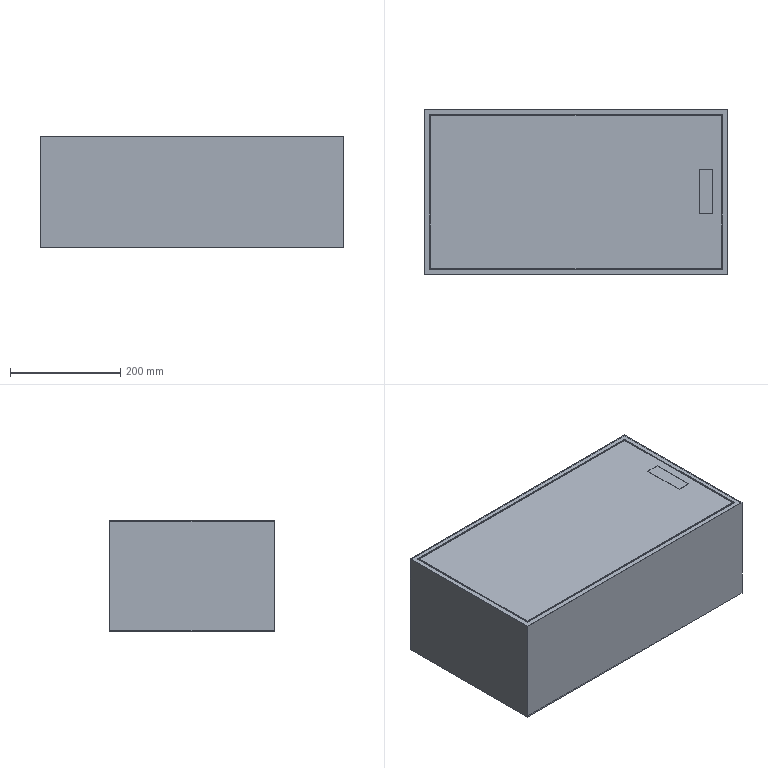Part | SolidWorks | features ICE 3, Extrusion 1, Shell 1 | 1 solid | 38 faces | box 550 x 300 x 201 mm | volume 911866 mm3 | plane 34 | cylinder 4 | commonest cylinder face diameters 22 x4
STEP:
#1=CARTESIAN_POINT('',(549.5,110.,154.));
#2=VERTEX_POINT('',#1);
#3=CARTESIAN_POINT('',(549.5,110.,132.));
#4=VERTEX_POINT('',#3);
#5=CARTESIAN_POINT('',(549.5,110.,143.));
#6=DIRECTION('',(1.,0.,0.));
#7=DIRECTION('',(0.,0.,-1.));
#8=AXIS2_PLACEMENT_3D('',#5,#6,#7);
#9=CIRCLE('',#8,11.);
#10=EDGE_CURVE('',#2,#4,#9,.T.);
#11=ORIENTED_EDGE('',*,*,#10,.F.);
#12=CARTESIAN_POINT('',(550.,110.,154.));
#13=VERTEX_POINT('',#12);
#14=CARTESIAN_POINT('',(549.5,110.,154.));
#15=DIRECTION('',(1.,0.,0.));
#16=VECTOR('',#15,1000.);
#17=LINE('',#14,#16);
#18=EDGE_CURVE('',#2,#13,#17,.T.);
#19=ORIENTED_EDGE('',*,*,#18,.T.);
#20=CARTESIAN_POINT('',(550.,110.,132.));
#21=VERTEX_POINT('',#20);
#22=CARTESIAN_POINT('',(550.,110.,143.));
#23=DIRECTION('',(1.,0.,0.));
#24=DIRECTION('',(0.,0.,-1.));
#25=AXIS2_PLACEMENT_3D('',#22,#23,#24);
#26=CIRCLE('',#25,11.);
#27=EDGE_CURVE('',#13,#21,#26,.T.);
#28=ORIENTED_EDGE('',*,*,#27,.T.);
#29=CARTESIAN_POINT('',(549.5,110.,132.));
#30=DIRECTION('',(1.,0.,0.));
#31=VECTOR('',#30,1000.);
#32=LINE('',#29,#31);
#33=EDGE_CURVE('',#4,#21,#32,.T.);
#34=ORIENTED_EDGE('',*,*,#33,.F.);
#35=EDGE_LOOP('',(#11,#19,#28,#34));
#36=FACE_OUTER_BOUND('',#35,.T.);
#37=CARTESIAN_POINT('',(549.5,110.,143.));
#38=DIRECTION('',(1.,0.,0.));
#39=DIRECTION('',(0.,0.,-1.));
#40=AXIS2_PLACEMENT_3D('',#37,#38,#39);
#41=CYLINDRICAL_SURFACE('',#40,11.);
#42=ADVANCED_FACE('',(#36),#41,.F.);
#43=CARTESIAN_POINT('',(549.5,110.,69.));
#44=VERTEX_POINT('',#43);
#45=CARTESIAN_POINT('',(549.5,110.,47.));
#46=VERTEX_POINT('',#45);
#47=CARTESIAN_POINT('',(549.5,110.,58.));
#48=DIRECTION('',(1.,0.,0.));
#49=DIRECTION('',(0.,0.,-1.));
#50=AXIS2_PLACEMENT_3D('',#47,#48,#49);
#51=CIRCLE('',#50,11.);
#52=EDGE_CURVE('',#44,#46,#51,.T.);
#53=ORIENTED_EDGE('',*,*,#52,.F.);
#54=CARTESIAN_POINT('',(550.,110.,69.));
#55=VERTEX_POINT('',#54);
#56=CARTESIAN_POINT('',(549.5,110.,69.));
#57=DIRECTION('',(1.,0.,0.));
#58=VECTOR('',#57,1000.);
#59=LINE('',#56,#58);
#60=EDGE_CURVE('',#44,#55,#59,.T.);
#61=ORIENTED_EDGE('',*,*,#60,.T.);
#62=CARTESIAN_POINT('',(550.,110.,47.));
#63=VERTEX_POINT('',#62);
#64=CARTESIAN_POINT('',(550.,110.,58.));
#65=DIRECTION('',(1.,0.,0.));
#66=DIRECTION('',(0.,0.,-1.));
#67=AXIS2_PLACEMENT_3D('',#64,#65,#66);
#68=CIRCLE('',#67,11.);
#69=EDGE_CURVE('',#55,#63,#68,.T.);
#70=ORIENTED_EDGE('',*,*,#69,.T.);
#71=CARTESIAN_POINT('',(549.5,110.,47.));
#72=DIRECTION('',(1.,0.,0.));
#73=VECTOR('',#72,1000.);
#74=LINE('',#71,#73);
#75=EDGE_CURVE('',#46,#63,#74,.T.);
#76=ORIENTED_EDGE('',*,*,#75,.F.);
#77=EDGE_LOOP('',(#53,#61,#70,#76));
#78=FACE_OUTER_BOUND('',#77,.T.);
#79=CARTESIAN_POINT('',(549.5,110.,58.));
#80=DIRECTION('',(1.,0.,0.));
#81=DIRECTION('',(0.,0.,-1.));
#82=AXIS2_PLACEMENT_3D('',#79,#80,#81);
#83=CYLINDRICAL_SURFACE('',#82,11.);
#84=ADVANCED_FACE('',(#78),#83,.F.);
#85=CARTESIAN_POINT('',(0.,300.,0.));
#86=VERTEX_POINT('',#85);
#87=CARTESIAN_POINT('',(0.,0.,0.));
#88=VERTEX_POINT('',#87);
#89=CARTESIAN_POINT('',(0.,0.,0.));
#90=DIRECTION('',(0.,-1.,0.));
#91=VECTOR('',#90,1000.);
#92=LINE('',#89,#91);
#93=EDGE_CURVE('',#86,#88,#92,.T.);
#94=ORIENTED_EDGE('',*,*,#93,.T.);
#95=CARTESIAN_POINT('',(0.,0.,201.));
#96=VERTEX_POINT('',#95);
#97=CARTESIAN_POINT('',(0.,0.,200.));
#98=DIRECTION('',(0.,0.,-1.));
#99=VECTOR('',#98,1000.);
#100=LINE('',#97,#99);
#101=EDGE_CURVE('',#96,#88,#100,.T.);
#102=ORIENTED_EDGE('',*,*,#101,.F.);
#103=CARTESIAN_POINT('',(0.,300.,201.));
#104=VERTEX_POINT('',#103);
#105=CARTESIAN_POINT('',(0.,300.,201.));
#106=DIRECTION('',(0.,-1.,0.));
#107=VECTOR('',#106,1000.);
#108=LINE('',#105,#107);
#109=EDGE_CURVE('',#104,#96,#108,.T.);
#110=ORIENTED_EDGE('',*,*,#109,.F.);
#111=CARTESIAN_POINT('',(0.,300.,200.));
#112=DIRECTION('',(0.,0.,-1.));
#113=VECTOR('',#112,1000.);
#114=LINE('',#111,#113);
#115=EDGE_CURVE('',#104,#86,#114,.T.);
#116=ORIENTED_EDGE('',*,*,#115,.T.);
#117=EDGE_LOOP('',(#94,#102,#110,#116));
#118=FACE_OUTER_BOUND('',#117,.T.);
#119=CARTESIAN_POINT('',(0.,0.,200.));
#120=DIRECTION('',(1.,0.,0.));
#121=DIRECTION('',(0.,0.,-1.));
#122=AXIS2_PLACEMENT_3D('',#119,#120,#121);
#123=PLANE('',#122);
#124=ADVANCED_FACE('',(#118),#123,.F.);
#125=CARTESIAN_POINT('',(550.,0.,0.));
#126=VERTEX_POINT('',#125);
#127=CARTESIAN_POINT('',(0.,0.,0.));
#128=DIRECTION('',(1.,0.,0.));
#129=VECTOR('',#128,1000.);
#130=LINE('',#127,#129);
#131=EDGE_CURVE('',#88,#126,#130,.T.);
#132=ORIENTED_EDGE('',*,*,#131,.T.);
#133=CARTESIAN_POINT('',(550.,0.,201.));
#134=VERTEX_POINT('',#133);
#135=CARTESIAN_POINT('',(550.,0.,200.));
#136=DIRECTION('',(0.,0.,-1.));
#137=VECTOR('',#136,1000.);
#138=LINE('',#135,#137);
#139=EDGE_CURVE('',#134,#126,#138,.T.);
#140=ORIENTED_EDGE('',*,*,#139,.F.);
#141=CARTESIAN_POINT('',(0.,0.,201.));
#142=DIRECTION('',(1.,0.,0.));
#143=VECTOR('',#142,1000.);
#144=LINE('',#141,#143);
#145=EDGE_CURVE('',#96,#134,#144,.T.);
#146=ORIENTED_EDGE('',*,*,#145,.F.);
#147=ORIENTED_EDGE('',*,*,#101,.T.);
#148=EDGE_LOOP('',(#132,#140,#146,#147));
#149=FACE_OUTER_BOUND('',#148,.T.);
#150=CARTESIAN_POINT('',(0.,0.,200.));
#151=DIRECTION('',(0.,1.,0.));
#152=DIRECTION('',(0.,0.,1.));
#153=AXIS2_PLACEMENT_3D('',#150,#151,#152);
#154=PLANE('',#153);
#155=ADVANCED_FACE('',(#149),#154,.F.);
#156=CARTESIAN_POINT('',(550.,240.,54.5));
#157=VERTEX_POINT('',#156);
#158=CARTESIAN_POINT('',(550.,240.,146.5));
#159=VERTEX_POINT('',#158);
#160=CARTESIAN_POINT('',(550.,240.,146.5));
#161=DIRECTION('',(0.,0.,1.));
#162=VECTOR('',#161,1000.);
#163=LINE('',#160,#162);
#164=EDGE_CURVE('',#157,#159,#163,.T.);
#165=ORIENTED_EDGE('',*,*,#164,.F.);
#166=CARTESIAN_POINT('',(550.,195.,54.5));
#167=VERTEX_POINT('',#166);
#168=CARTESIAN_POINT('',(550.,240.,54.5));
#169=DIRECTION('',(0.,1.,0.));
#170=VECTOR('',#169,1000.);
#171=LINE('',#168,#170);
#172=EDGE_CURVE('',#167,#157,#171,.T.);
#173=ORIENTED_EDGE('',*,*,#172,.F.);
#174=CARTESIAN_POINT('',(550.,195.,146.5));
#175=VERTEX_POINT('',#174);
#176=CARTESIAN_POINT('',(550.,195.,146.5));
#177=DIRECTION('',(0.,0.,-1.));
#178=VECTOR('',#177,1000.);
#179=LINE('',#176,#178);
#180=EDGE_CURVE('',#175,#167,#179,.T.);
#181=ORIENTED_EDGE('',*,*,#180,.F.);
#182=CARTESIAN_POINT('',(550.,240.,146.5));
#183=DIRECTION('',(0.,-1.,0.));
#184=VECTOR('',#183,1000.);
#185=LINE('',#182,#184);
#186=EDGE_CURVE('',#159,#175,#185,.T.);
#187=ORIENTED_EDGE('',*,*,#186,.F.);
#188=EDGE_LOOP('',(#165,#173,#181,#187));
#189=FACE_BOUND('',#188,.T.);
#190=CARTESIAN_POINT('',(550.,110.,143.));
#191=DIRECTION('',(1.,0.,0.));
#192=DIRECTION('',(0.,0.,-1.));
#193=AXIS2_PLACEMENT_3D('',#190,#191,#192);
#194=CIRCLE('',#193,11.);
#195=EDGE_CURVE('',#21,#13,#194,.T.);
#196=ORIENTED_EDGE('',*,*,#195,.F.);
#197=ORIENTED_EDGE('',*,*,#27,.F.);
#198=EDGE_LOOP('',(#196,#197));
#199=FACE_BOUND('',#198,.T.);
#200=CARTESIAN_POINT('',(550.,110.,58.));
#201=DIRECTION('',(1.,0.,0.));
#202=DIRECTION('',(0.,0.,-1.));
#203=AXIS2_PLACEMENT_3D('',#200,#201,#202);
#204=CIRCLE('',#203,11.);
#205=EDGE_CURVE('',#63,#55,#204,.T.);
#206=ORIENTED_EDGE('',*,*,#205,.F.);
#207=ORIENTED_EDGE('',*,*,#69,.F.);
#208=EDGE_LOOP('',(#206,#207));
#209=FACE_BOUND('',#208,.T.);
#210=CARTESIAN_POINT('',(550.,300.,0.));
#211=VERTEX_POINT('',#210);
#212=CARTESIAN_POINT('',(550.,0.,0.));
#213=DIRECTION('',(0.,1.,0.));
#214=VECTOR('',#213,1000.);
#215=LINE('',#212,#214);
#216=EDGE_CURVE('',#126,#211,#215,.T.);
#217=ORIENTED_EDGE('',*,*,#216,.T.);
#218=CARTESIAN_POINT('',(550.,300.,201.));
#219=VERTEX_POINT('',#218);
#220=CARTESIAN_POINT('',(550.,300.,200.));
#221=DIRECTION('',(0.,0.,-1.));
#222=VECTOR('',#221,1000.);
#223=LINE('',#220,#222);
#224=EDGE_CURVE('',#219,#211,#223,.T.);
#225=ORIENTED_EDGE('',*,*,#224,.F.);
#226=CARTESIAN_POINT('',(550.,0.,201.));
#227=DIRECTION('',(0.,1.,0.));
#228=VECTOR('',#227,1000.);
#229=LINE('',#226,#228);
#230=EDGE_CURVE('',#134,#219,#229,.T.);
#231=ORIENTED_EDGE('',*,*,#230,.F.);
#232=ORIENTED_EDGE('',*,*,#139,.T.);
#233=EDGE_LOOP('',(#217,#225,#231,#232));
#234=FACE_OUTER_BOUND('',#233,.T.);
#235=CARTESIAN_POINT('',(550.,0.,200.));
#236=DIRECTION('',(-1.,0.,0.));
#237=DIRECTION('',(0.,0.,1.));
#238=AXIS2_PLACEMENT_3D('',#235,#236,#237);
#239=PLANE('',#238);
#240=ADVANCED_FACE('',(#189,#199,#209,#234),#239,.F.);
#241=CARTESIAN_POINT('',(0.,300.,0.));
#242=DIRECTION('',(-1.,0.,0.));
#243=VECTOR('',#242,1000.);
#244=LINE('',#241,#243);
#245=EDGE_CURVE('',#211,#86,#244,.T.);
#246=ORIENTED_EDGE('',*,*,#245,.T.);
#247=ORIENTED_EDGE('',*,*,#115,.F.);
#248=CARTESIAN_POINT('',(550.,300.,201.));
#249=DIRECTION('',(-1.,0.,0.));
#250=VECTOR('',#249,1000.);
#251=LINE('',#248,#250);
#252=EDGE_CURVE('',#219,#104,#251,.T.);
#253=ORIENTED_EDGE('',*,*,#252,.F.);
#254=ORIENTED_EDGE('',*,*,#224,.T.);
#255=EDGE_LOOP('',(#246,#247,#253,#254));
#256=FACE_OUTER_BOUND('',#255,.T.);
#257=CARTESIAN_POINT('',(0.,300.,200.));
#258=DIRECTION('',(0.,-1.,0.));
#259=DIRECTION('',(0.,0.,-1.));
#260=AXIS2_PLACEMENT_3D('',#257,#258,#259);
#261=PLANE('',#260);
#262=ADVANCED_FACE('',(#256),#261,.F.);
#263=ORIENTED_EDGE('',*,*,#93,.F.);
#264=ORIENTED_EDGE('',*,*,#245,.F.);
#265=ORIENTED_EDGE('',*,*,#216,.F.);
#266=ORIENTED_EDGE('',*,*,#131,.F.);
#267=EDGE_LOOP('',(#263,#264,#265,#266));
#268=FACE_OUTER_BOUND('',#267,.T.);
#269=CARTESIAN_POINT('',(0.,0.,0.));
#270=DIRECTION('',(0.,0.,-1.));
#271=DIRECTION('',(-1.,0.,0.));
#272=AXIS2_PLACEMENT_3D('',#269,#270,#271);
#273=PLANE('',#272);
#274=ADVANCED_FACE('',(#268),#273,.T.);
#275=CARTESIAN_POINT('',(540.,290.,201.));
#276=VERTEX_POINT('',#275);
#277=CARTESIAN_POINT('',(10.,290.,201.));
#278=VERTEX_POINT('',#277);
#279=CARTESIAN_POINT('',(0.,290.,201.));
#280=DIRECTION('',(-1.,0.,0.));
#281=VECTOR('',#280,1000.);
#282=LINE('',#279,#281);
#283=EDGE_CURVE('',#276,#278,#282,.T.);
#284=ORIENTED_EDGE('',*,*,#283,.F.);
#285=CARTESIAN_POINT('',(540.,10.,201.));
#286=VERTEX_POINT('',#285);
#287=CARTESIAN_POINT('',(540.,0.,201.));
#288=DIRECTION('',(0.,1.,0.));
#289=VECTOR('',#288,1000.);
#290=LINE('',#287,#289);
#291=EDGE_CURVE('',#286,#276,#290,.T.);
#292=ORIENTED_EDGE('',*,*,#291,.F.);
#293=CARTESIAN_POINT('',(10.,10.,201.));
#294=VERTEX_POINT('',#293);
#295=CARTESIAN_POINT('',(0.,10.,201.));
#296=DIRECTION('',(1.,0.,0.));
#297=VECTOR('',#296,1000.);
#298=LINE('',#295,#297);
#299=EDGE_CURVE('',#294,#286,#298,.T.);
#300=ORIENTED_EDGE('',*,*,#299,.F.);
#301=CARTESIAN_POINT('',(10.,0.,201.));
#302=DIRECTION('',(0.,-1.,0.));
#303=VECTOR('',#302,1000.);
#304=LINE('',#301,#303);
#305=EDGE_CURVE('',#278,#294,#304,.T.);
#306=ORIENTED_EDGE('',*,*,#305,.F.);
#307=EDGE_LOOP('',(#284,#292,#300,#306));
#308=FACE_BOUND('',#307,.T.);
#309=ORIENTED_EDGE('',*,*,#252,.T.);
#310=ORIENTED_EDGE('',*,*,#109,.T.);
#311=ORIENTED_EDGE('',*,*,#145,.T.);
#312=ORIENTED_EDGE('',*,*,#230,.T.);
#313=EDGE_LOOP('',(#309,#310,#311,#312));
#314=FACE_OUTER_BOUND('',#313,.T.);
#315=CARTESIAN_POINT('',(0.,0.,201.));
#316=DIRECTION('',(0.,0.,1.));
#317=DIRECTION('',(1.,0.,0.));
#318=AXIS2_PLACEMENT_3D('',#315,#316,#317);
#319=PLANE('',#318);
#320=ADVANCED_FACE('',(#308,#314),#319,.T.);
#321=ORIENTED_EDGE('',*,*,#283,.T.);
#322=CARTESIAN_POINT('',(10.,290.,200.5));
#323=VERTEX_POINT('',#322);
#324=CARTESIAN_POINT('',(10.,290.,200.5));
#325=DIRECTION('',(0.,0.,1.));
#326=VECTOR('',#325,1000.);
#327=LINE('',#324,#326);
#328=EDGE_CURVE('',#323,#278,#327,.T.);
#329=ORIENTED_EDGE('',*,*,#328,.F.);
#330=CARTESIAN_POINT('',(540.,290.,200.5));
#331=VERTEX_POINT('',#330);
#332=CARTESIAN_POINT('',(0.,290.,200.5));
#333=DIRECTION('',(-1.,0.,0.));
#334=VECTOR('',#333,1000.);
#335=LINE('',#332,#334);
#336=EDGE_CURVE('',#331,#323,#335,.T.);
#337=ORIENTED_EDGE('',*,*,#336,.F.);
#338=CARTESIAN_POINT('',(540.,290.,200.5));
#339=DIRECTION('',(0.,0.,1.));
#340=VECTOR('',#339,1000.);
#341=LINE('',#338,#340);
#342=EDGE_CURVE('',#331,#276,#341,.T.);
#343=ORIENTED_EDGE('',*,*,#342,.T.);
#344=EDGE_LOOP('',(#321,#329,#337,#343));
#345=FACE_OUTER_BOUND('',#344,.T.);
#346=CARTESIAN_POINT('',(0.,290.,200.5));
#347=DIRECTION('',(0.,1.,0.));
#348=DIRECTION('',(0.,0.,1.));
#349=AXIS2_PLACEMENT_3D('',#346,#347,#348);
#350=PLANE('',#349);
#351=ADVANCED_FACE('',(#345),#350,.F.);
#352=ORIENTED_EDGE('',*,*,#291,.T.);
#353=ORIENTED_EDGE('',*,*,#342,.F.);
#354=CARTESIAN_POINT('',(540.,10.,200.5));
#355=VERTEX_POINT('',#354);
#356=CARTESIAN_POINT('',(540.,0.,200.5));
#357=DIRECTION('',(0.,1.,0.));
#358=VECTOR('',#357,1000.);
#359=LINE('',#356,#358);
#360=EDGE_CURVE('',#355,#331,#359,.T.);
#361=ORIENTED_EDGE('',*,*,#360,.F.);
#362=CARTESIAN_POINT('',(540.,10.,200.5));
#363=DIRECTION('',(0.,0.,1.));
#364=VECTOR('',#363,1000.);
#365=LINE('',#362,#364);
#366=EDGE_CURVE('',#355,#286,#365,.T.);
#367=ORIENTED_EDGE('',*,*,#366,.T.);
#368=EDGE_LOOP('',(#352,#353,#361,#367));
#369=FACE_OUTER_BOUND('',#368,.T.);
#370=CARTESIAN_POINT('',(540.,0.,200.5));
#371=DIRECTION('',(1.,0.,0.));
#372=DIRECTION('',(0.,0.,-1.));
#373=AXIS2_PLACEMENT_3D('',#370,#371,#372);
#374=PLANE('',#373);
#375=ADVANCED_FACE('',(#369),#374,.F.);
#376=ORIENTED_EDGE('',*,*,#299,.T.);
#377=ORIENTED_EDGE('',*,*,#366,.F.);
#378=CARTESIAN_POINT('',(10.,10.,200.5));
#379=VERTEX_POINT('',#378);
#380=CARTESIAN_POINT('',(0.,10.,200.5));
#381=DIRECTION('',(1.,0.,0.));
#382=VECTOR('',#381,1000.);
#383=LINE('',#380,#382);
#384=EDGE_CURVE('',#379,#355,#383,.T.);
#385=ORIENTED_EDGE('',*,*,#384,.F.);
#386=CARTESIAN_POINT('',(10.,10.,200.5));
#387=DIRECTION('',(0.,0.,1.));
#388=VECTOR('',#387,1000.);
#389=LINE('',#386,#388);
#390=EDGE_CURVE('',#379,#294,#389,.T.);
#391=ORIENTED_EDGE('',*,*,#390,.T.);
#392=EDGE_LOOP('',(#376,#377,#385,#391));
#393=FACE_OUTER_BOUND('',#392,.T.);
#394=CARTESIAN_POINT('',(0.,10.,200.5));
#395=DIRECTION('',(0.,-1.,0.));
#396=DIRECTION('',(0.,0.,-1.));
#397=AXIS2_PLACEMENT_3D('',#394,#395,#396);
#398=PLANE('',#397);
#399=ADVANCED_FACE('',(#393),#398,.F.);
#400=CARTESIAN_POINT('',(538.,12.,201.));
#401=VERTEX_POINT('',#400);
#402=CARTESIAN_POINT('',(538.,288.,201.));
#403=VERTEX_POINT('',#402);
#404=CARTESIAN_POINT('',(538.,0.,201.));
#405=DIRECTION('',(0.,1.,0.));
#406=VECTOR('',#405,1000.);
#407=LINE('',#404,#406);
#408=EDGE_CURVE('',#401,#403,#407,.T.);
#409=ORIENTED_EDGE('',*,*,#408,.F.);
#410=CARTESIAN_POINT('',(538.,12.,200.5));
#411=VERTEX_POINT('',#410);
#412=CARTESIAN_POINT('',(538.,12.,200.5));
#413=DIRECTION('',(0.,0.,1.));
#414=VECTOR('',#413,1000.);
#415=LINE('',#412,#414);
#416=EDGE_CURVE('',#411,#401,#415,.T.);
#417=ORIENTED_EDGE('',*,*,#416,.F.);
#418=CARTESIAN_POINT('',(538.,288.,200.5));
#419=VERTEX_POINT('',#418);
#420=CARTESIAN_POINT('',(538.,0.,200.5));
#421=DIRECTION('',(0.,1.,0.));
#422=VECTOR('',#421,1000.);
#423=LINE('',#420,#422);
#424=EDGE_CURVE('',#411,#419,#423,.T.);
#425=ORIENTED_EDGE('',*,*,#424,.T.);
#426=CARTESIAN_POINT('',(538.,288.,200.5));
#427=DIRECTION('',(0.,0.,1.));
#428=VECTOR('',#427,1000.);
#429=LINE('',#426,#428);
#430=EDGE_CURVE('',#419,#403,#429,.T.);
#431=ORIENTED_EDGE('',*,*,#430,.T.);
#432=EDGE_LOOP('',(#409,#417,#425,#431));
#433=FACE_OUTER_BOUND('',#432,.T.);
#434=CARTESIAN_POINT('',(538.,0.,200.5));
#435=DIRECTION('',(1.,0.,0.));
#436=DIRECTION('',(0.,0.,-1.));
#437=AXIS2_PLACEMENT_3D('',#434,#435,#436);
#438=PLANE('',#437);
#439=ADVANCED_FACE('',(#433),#438,.T.);
#440=CARTESIAN_POINT('',(12.,288.,201.));
#441=VERTEX_POINT('',#440);
#442=CARTESIAN_POINT('',(0.,288.,201.));
#443=DIRECTION('',(-1.,0.,0.));
#444=VECTOR('',#443,1000.);
#445=LINE('',#442,#444);
#446=EDGE_CURVE('',#403,#441,#445,.T.);
#447=ORIENTED_EDGE('',*,*,#446,.F.);
#448=ORIENTED_EDGE('',*,*,#430,.F.);
#449=CARTESIAN_POINT('',(12.,288.,200.5));
#450=VERTEX_POINT('',#449);
#451=CARTESIAN_POINT('',(0.,288.,200.5));
#452=DIRECTION('',(-1.,0.,0.));
#453=VECTOR('',#452,1000.);
#454=LINE('',#451,#453);
#455=EDGE_CURVE('',#419,#450,#454,.T.);
#456=ORIENTED_EDGE('',*,*,#455,.T.);
#457=CARTESIAN_POINT('',(12.,288.,200.5));
#458=DIRECTION('',(0.,0.,1.));
#459=VECTOR('',#458,1000.);
#460=LINE('',#457,#459);
#461=EDGE_CURVE('',#450,#441,#460,.T.);
#462=ORIENTED_EDGE('',*,*,#461,.T.);
#463=EDGE_LOOP('',(#447,#448,#456,#462));
#464=FACE_OUTER_BOUND('',#463,.T.);
#465=CARTESIAN_POINT('',(0.,288.,200.5));
#466=DIRECTION('',(0.,1.,0.));
#467=DIRECTION('',(0.,0.,1.));
#468=AXIS2_PLACEMENT_3D('',#465,#466,#467);
#469=PLANE('',#468);
#470=ADVANCED_FACE('',(#464),#469,.T.);
#471=CARTESIAN_POINT('',(12.,12.,201.));
#472=VERTEX_POINT('',#471);
#473=CARTESIAN_POINT('',(12.,0.,201.));
#474=DIRECTION('',(0.,-1.,0.));
#475=VECTOR('',#474,1000.);
#476=LINE('',#473,#475);
#477=EDGE_CURVE('',#441,#472,#476,.T.);
#478=ORIENTED_EDGE('',*,*,#477,.F.);
#479=ORIENTED_EDGE('',*,*,#461,.F.);
#480=CARTESIAN_POINT('',(12.,12.,200.5));
#481=VERTEX_POINT('',#480);
#482=CARTESIAN_POINT('',(12.,0.,200.5));
#483=DIRECTION('',(0.,-1.,0.));
#484=VECTOR('',#483,1000.);
#485=LINE('',#482,#484);
#486=EDGE_CURVE('',#450,#481,#485,.T.);
#487=ORIENTED_EDGE('',*,*,#486,.T.);
#488=CARTESIAN_POINT('',(12.,12.,200.5));
#489=DIRECTION('',(0.,0.,1.));
#490=VECTOR('',#489,1000.);
#491=LINE('',#488,#490);
#492=EDGE_CURVE('',#481,#472,#491,.T.);
#493=ORIENTED_EDGE('',*,*,#492,.T.);
#494=EDGE_LOOP('',(#478,#479,#487,#493));
#495=FACE_OUTER_BOUND('',#494,.T.);
#496=CARTESIAN_POINT('',(12.,0.,200.5));
#497=DIRECTION('',(-1.,0.,0.));
#498=DIRECTION('',(0.,0.,1.));
#499=AXIS2_PLACEMENT_3D('',#496,#497,#498);
#500=PLANE('',#499);
#501=ADVANCED_FACE('',(#495),#500,.T.);
#502=CARTESIAN_POINT('',(0.,12.,201.));
#503=DIRECTION('',(1.,0.,0.));
#504=VECTOR('',#503,1000.);
#505=LINE('',#502,#504);
#506=EDGE_CURVE('',#472,#401,#505,.T.);
#507=ORIENTED_EDGE('',*,*,#506,.F.);
#508=ORIENTED_EDGE('',*,*,#492,.F.);
#509=CARTESIAN_POINT('',(0.,12.,200.5));
#510=DIRECTION('',(1.,0.,0.));
#511=VECTOR('',#510,1000.);
#512=LINE('',#509,#511);
#513=EDGE_CURVE('',#481,#411,#512,.T.);
#514=ORIENTED_EDGE('',*,*,#513,.T.);
#515=ORIENTED_EDGE('',*,*,#416,.T.);
#516=EDGE_LOOP('',(#507,#508,#514,#515));
#517=FACE_OUTER_BOUND('',#516,.T.);
#518=CARTESIAN_POINT('',(0.,12.,200.5));
#519=DIRECTION('',(0.,-1.,0.));
#520=DIRECTION('',(1.,0.,0.));
#521=AXIS2_PLACEMENT_3D('',#518,#519,#520);
#522=PLANE('',#521);
#523=ADVANCED_FACE('',(#517),#522,.T.);
#524=ORIENTED_EDGE('',*,*,#305,.T.);
#525=ORIENTED_EDGE('',*,*,#390,.F.);
#526=CARTESIAN_POINT('',(10.,0.,200.5));
#527=DIRECTION('',(0.,-1.,0.));
#528=VECTOR('',#527,1000.);
#529=LINE('',#526,#528);
#530=EDGE_CURVE('',#323,#379,#529,.T.);
#531=ORIENTED_EDGE('',*,*,#530,.F.);
#532=ORIENTED_EDGE('',*,*,#328,.T.);
#533=EDGE_LOOP('',(#524,#525,#531,#532));
#534=FACE_OUTER_BOUND('',#533,.T.);
#535=CARTESIAN_POINT('',(10.,0.,200.5));
#536=DIRECTION('',(-1.,0.,0.));
#537=DIRECTION('',(0.,0.,1.));
#538=AXIS2_PLACEMENT_3D('',#535,#536,#537);
#539=PLANE('',#538);
#540=ADVANCED_FACE('',(#534),#539,.F.);
#541=ORIENTED_EDGE('',*,*,#424,.F.);
#542=ORIENTED_EDGE('',*,*,#513,.F.);
#543=ORIENTED_EDGE('',*,*,#486,.F.);
#544=ORIENTED_EDGE('',*,*,#455,.F.);
#545=EDGE_LOOP('',(#541,#542,#543,#544));
#546=FACE_BOUND('',#545,.T.);
#547=ORIENTED_EDGE('',*,*,#336,.T.);
#548=ORIENTED_EDGE('',*,*,#530,.T.);
#549=ORIENTED_EDGE('',*,*,#384,.T.);
#550=ORIENTED_EDGE('',*,*,#360,.T.);
#551=EDGE_LOOP('',(#547,#548,#549,#550));
#552=FACE_OUTER_BOUND('',#551,.T.);
#553=CARTESIAN_POINT('',(0.,0.,200.5));
#554=DIRECTION('',(0.,0.,1.));
#555=DIRECTION('',(1.,0.,0.));
#556=AXIS2_PLACEMENT_3D('',#553,#554,#555);
#557=PLANE('',#556);
#558=ADVANCED_FACE('',(#546,#552),#557,.T.);
#559=CARTESIAN_POINT('',(499.,110.,201.));
#560=VERTEX_POINT('',#559);
#561=CARTESIAN_POINT('',(523.,110.,201.));
#562=VERTEX_POINT('',#561);
#563=CARTESIAN_POINT('',(0.,110.,201.));
#564=DIRECTION('',(1.,0.,0.));
#565=VECTOR('',#564,1000.);
#566=LINE('',#563,#565);
#567=EDGE_CURVE('',#560,#562,#566,.T.);
#568=ORIENTED_EDGE('',*,*,#567,.F.);
#569=CARTESIAN_POINT('',(499.,190.,201.));
#570=VERTEX_POINT('',#569);
#571=CARTESIAN_POINT('',(499.,0.,201.));
#572=DIRECTION('',(0.,1.,0.));
#573=VECTOR('',#572,1000.);
#574=LINE('',#571,#573);
#575=EDGE_CURVE('',#560,#570,#574,.T.);
#576=ORIENTED_EDGE('',*,*,#575,.T.);
#577=CARTESIAN_POINT('',(523.,190.,201.));
#578=VERTEX_POINT('',#577);
#579=CARTESIAN_POINT('',(0.,190.,201.));
#580=DIRECTION('',(1.,0.,0.));
#581=VECTOR('',#580,1000.);
#582=LINE('',#579,#581);
#583=EDGE_CURVE('',#570,#578,#582,.T.);
#584=ORIENTED_EDGE('',*,*,#583,.T.);
#585=CARTESIAN_POINT('',(523.,0.,201.));
#586=DIRECTION('',(0.,1.,0.));
#587=VECTOR('',#586,1000.);
#588=LINE('',#585,#587);
#589=EDGE_CURVE('',#562,#578,#588,.T.);
#590=ORIENTED_EDGE('',*,*,#589,.F.);
#591=EDGE_LOOP('',(#568,#576,#584,#590));
#592=FACE_BOUND('',#591,.T.);
#593=ORIENTED_EDGE('',*,*,#506,.T.);
#594=ORIENTED_EDGE('',*,*,#408,.T.);
#595=ORIENTED_EDGE('',*,*,#446,.T.);
#596=ORIENTED_EDGE('',*,*,#477,.T.);
#597=EDGE_LOOP('',(#593,#594,#595,#596));
#598=FACE_OUTER_BOUND('',#597,.T.);
#599=CARTESIAN_POINT('',(0.,0.,201.));
#600=DIRECTION('',(0.,0.,1.));
#601=DIRECTION('',(1.,0.,0.));
#602=AXIS2_PLACEMENT_3D('',#599,#600,#601);
#603=PLANE('',#602);
#604=ADVANCED_FACE('',(#592,#598),#603,.T.);
#605=ORIENTED_EDGE('',*,*,#567,.T.);
#606=CARTESIAN_POINT('',(523.,110.,200.5));
#607=VERTEX_POINT('',#606);
#608=CARTESIAN_POINT('',(523.,110.,200.5));
#609=DIRECTION('',(0.,0.,1.));
#610=VECTOR('',#609,1000.);
#611=LINE('',#608,#610);
#612=EDGE_CURVE('',#607,#562,#611,.T.);
#613=ORIENTED_EDGE('',*,*,#612,.F.);
#614=CARTESIAN_POINT('',(499.,110.,200.5));
#615=VERTEX_POINT('',#614);
#616=CARTESIAN_POINT('',(0.,110.,200.5));
#617=DIRECTION('',(1.,0.,0.));
#618=VECTOR('',#617,1000.);
#619=LINE('',#616,#618);
#620=EDGE_CURVE('',#615,#607,#619,.T.);
#621=ORIENTED_EDGE('',*,*,#620,.F.);
#622=CARTESIAN_POINT('',(499.,110.,200.5));
#623=DIRECTION('',(0.,0.,1.));
#624=VECTOR('',#623,1000.);
#625=LINE('',#622,#624);
#626=EDGE_CURVE('',#615,#560,#625,.T.);
#627=ORIENTED_EDGE('',*,*,#626,.T.);
#628=EDGE_LOOP('',(#605,#613,#621,#627));
#629=FACE_OUTER_BOUND('',#628,.T.);
#630=CARTESIAN_POINT('',(0.,110.,200.5));
#631=DIRECTION('',(0.,-1.,0.));
#632=DIRECTION('',(0.,0.,-1.));
#633=AXIS2_PLACEMENT_3D('',#630,#631,#632);
#634=PLANE('',#633);
#635=ADVANCED_FACE('',(#629),#634,.F.);
#636=ORIENTED_EDGE('',*,*,#575,.F.);
#637=ORIENTED_EDGE('',*,*,#626,.F.);
#638=CARTESIAN_POINT('',(499.,190.,200.5));
#639=VERTEX_POINT('',#638);
#640=CARTESIAN_POINT('',(499.,0.,200.5));
#641=DIRECTION('',(0.,1.,0.));
#642=VECTOR('',#641,1000.);
#643=LINE('',#640,#642);
#644=EDGE_CURVE('',#615,#639,#643,.T.);
#645=ORIENTED_EDGE('',*,*,#644,.T.);
#646=CARTESIAN_POINT('',(499.,190.,200.5));
#647=DIRECTION('',(0.,0.,1.));
#648=VECTOR('',#647,1000.);
#649=LINE('',#646,#648);
#650=EDGE_CURVE('',#639,#570,#649,.T.);
#651=ORIENTED_EDGE('',*,*,#650,.T.);
#652=EDGE_LOOP('',(#636,#637,#645,#651));
#653=FACE_OUTER_BOUND('',#652,.T.);
#654=CARTESIAN_POINT('',(499.,0.,200.5));
#655=DIRECTION('',(1.,0.,0.));
#656=DIRECTION('',(0.,0.,-1.));
#657=AXIS2_PLACEMENT_3D('',#654,#655,#656);
#658=PLANE('',#657);
#659=ADVANCED_FACE('',(#653),#658,.T.);
#660=ORIENTED_EDGE('',*,*,#583,.F.);
#661=ORIENTED_EDGE('',*,*,#650,.F.);
#662=CARTESIAN_POINT('',(523.,190.,200.5));
#663=VERTEX_POINT('',#662);
#664=CARTESIAN_POINT('',(0.,190.,200.5));
#665=DIRECTION('',(1.,0.,0.));
#666=VECTOR('',#665,1000.);
#667=LINE('',#664,#666);
#668=EDGE_CURVE('',#639,#663,#667,.T.);
#669=ORIENTED_EDGE('',*,*,#668,.T.);
#670=CARTESIAN_POINT('',(523.,190.,200.5));
#671=DIRECTION('',(0.,0.,1.));
#672=VECTOR('',#671,1000.);
#673=LINE('',#670,#672);
#674=EDGE_CURVE('',#663,#578,#673,.T.);
#675=ORIENTED_EDGE('',*,*,#674,.T.);
#676=EDGE_LOOP('',(#660,#661,#669,#675));
#677=FACE_OUTER_BOUND('',#676,.T.);
#678=CARTESIAN_POINT('',(0.,190.,200.5));
#679=DIRECTION('',(0.,-1.,0.));
#680=DIRECTION('',(0.,0.,-1.));
#681=AXIS2_PLACEMENT_3D('',#678,#679,#680);
#682=PLANE('',#681);
#683=ADVANCED_FACE('',(#677),#682,.T.);
#684=ORIENTED_EDGE('',*,*,#589,.T.);
#685=ORIENTED_EDGE('',*,*,#674,.F.);
#686=CARTESIAN_POINT('',(523.,0.,200.5));
#687=DIRECTION('',(0.,1.,0.));
#688=VECTOR('',#687,1000.);
#689=LINE('',#686,#688);
#690=EDGE_CURVE('',#607,#663,#689,.T.);
#691=ORIENTED_EDGE('',*,*,#690,.F.);
#692=ORIENTED_EDGE('',*,*,#612,.T.);
#693=EDGE_LOOP('',(#684,#685,#691,#692));
#694=FACE_OUTER_BOUND('',#693,.T.);
#695=CARTESIAN_POINT('',(523.,0.,200.5));
#696=DIRECTION('',(1.,0.,0.));
#697=DIRECTION('',(0.,0.,-1.));
#698=AXIS2_PLACEMENT_3D('',#695,#696,#697);
#699=PLANE('',#698);
#700=ADVANCED_FACE('',(#694),#699,.F.);
#701=ORIENTED_EDGE('',*,*,#620,.T.);
#702=ORIENTED_EDGE('',*,*,#690,.T.);
#703=ORIENTED_EDGE('',*,*,#668,.F.);
#704=ORIENTED_EDGE('',*,*,#644,.F.);
#705=EDGE_LOOP('',(#701,#702,#703,#704));
#706=FACE_OUTER_BOUND('',#705,.T.);
#707=CARTESIAN_POINT('',(0.,0.,200.5));
#708=DIRECTION('',(0.,0.,1.));
#709=DIRECTION('',(1.,0.,0.));
#710=AXIS2_PLACEMENT_3D('',#707,#708,#709);
#711=PLANE('',#710);
#712=ADVANCED_FACE('',(#706),#711,.T.);
#713=ORIENTED_EDGE('',*,*,#60,.F.);
#714=CARTESIAN_POINT('',(549.5,110.,58.));
#715=DIRECTION('',(1.,0.,0.));
#716=DIRECTION('',(0.,0.,-1.));
#717=AXIS2_PLACEMENT_3D('',#714,#715,#716);
#718=CIRCLE('',#717,11.);
#719=EDGE_CURVE('',#46,#44,#718,.T.);
#720=ORIENTED_EDGE('',*,*,#719,.F.);
#721=ORIENTED_EDGE('',*,*,#75,.T.);
#722=ORIENTED_EDGE('',*,*,#205,.T.);
#723=EDGE_LOOP('',(#713,#720,#721,#722));
#724=FACE_OUTER_BOUND('',#723,.T.);
#725=CARTESIAN_POINT('',(549.5,110.,58.));
#726=DIRECTION('',(1.,0.,0.));
#727=DIRECTION('',(0.,0.,-1.));
#728=AXIS2_PLACEMENT_3D('',#725,#726,#727);
#729=CYLINDRICAL_SURFACE('',#728,11.);
#730=ADVANCED_FACE('',(#724),#729,.F.);
#731=ORIENTED_EDGE('',*,*,#719,.T.);
#732=ORIENTED_EDGE('',*,*,#52,.T.);
#733=EDGE_LOOP('',(#731,#732));
#734=FACE_OUTER_BOUND('',#733,.T.);
#735=CARTESIAN_POINT('',(549.5,110.,58.));
#736=DIRECTION('',(1.,0.,0.));
#737=DIRECTION('',(0.,0.,-1.));
#738=AXIS2_PLACEMENT_3D('',#735,#736,#737);
#739=PLANE('',#738);
#740=ADVANCED_FACE('',(#734),#739,.T.);
#741=ORIENTED_EDGE('',*,*,#18,.F.);
#742=CARTESIAN_POINT('',(549.5,110.,143.));
#743=DIRECTION('',(1.,0.,0.));
#744=DIRECTION('',(0.,0.,-1.));
#745=AXIS2_PLACEMENT_3D('',#742,#743,#744);
#746=CIRCLE('',#745,11.);
#747=EDGE_CURVE('',#4,#2,#746,.T.);
#748=ORIENTED_EDGE('',*,*,#747,.F.);
#749=ORIENTED_EDGE('',*,*,#33,.T.);
#750=ORIENTED_EDGE('',*,*,#195,.T.);
#751=EDGE_LOOP('',(#741,#748,#749,#750));
#752=FACE_OUTER_BOUND('',#751,.T.);
#753=CARTESIAN_POINT('',(549.5,110.,143.));
#754=DIRECTION('',(1.,0.,0.));
#755=DIRECTION('',(0.,0.,-1.));
#756=AXIS2_PLACEMENT_3D('',#753,#754,#755);
#757=CYLINDRICAL_SURFACE('',#756,11.);
#758=ADVANCED_FACE('',(#752),#757,.F.);
#759=ORIENTED_EDGE('',*,*,#747,.T.);
#760=ORIENTED_EDGE('',*,*,#10,.T.);
#761=EDGE_LOOP('',(#759,#760));
#762=FACE_OUTER_BOUND('',#761,.T.);
#763=CARTESIAN_POINT('',(549.5,110.,143.));
#764=DIRECTION('',(1.,0.,0.));
#765=DIRECTION('',(0.,0.,-1.));
#766=AXIS2_PLACEMENT_3D('',#763,#764,#765);
#767=PLANE('',#766);
#768=ADVANCED_FACE('',(#762),#767,.T.);
#769=ORIENTED_EDGE('',*,*,#172,.T.);
#770=CARTESIAN_POINT('',(549.5,240.,54.5));
#771=VERTEX_POINT('',#770);
#772=CARTESIAN_POINT('',(549.5,240.,54.5));
#773=DIRECTION('',(1.,0.,0.));
#774=VECTOR('',#773,1000.);
#775=LINE('',#772,#774);
#776=EDGE_CURVE('',#771,#157,#775,.T.);
#777=ORIENTED_EDGE('',*,*,#776,.F.);
#778=CARTESIAN_POINT('',(549.5,195.,54.5));
#779=VERTEX_POINT('',#778);
#780=CARTESIAN_POINT('',(549.5,240.,54.5));
#781=DIRECTION('',(0.,1.,0.));
#782=VECTOR('',#781,1000.);
#783=LINE('',#780,#782);
#784=EDGE_CURVE('',#779,#771,#783,.T.);
#785=ORIENTED_EDGE('',*,*,#784,.F.);
#786=CARTESIAN_POINT('',(549.5,195.,54.5));
#787=DIRECTION('',(1.,0.,0.));
#788=VECTOR('',#787,1000.);
#789=LINE('',#786,#788);
#790=EDGE_CURVE('',#779,#167,#789,.T.);
#791=ORIENTED_EDGE('',*,*,#790,.T.);
#792=EDGE_LOOP('',(#769,#777,#785,#791));
#793=FACE_OUTER_BOUND('',#792,.T.);
#794=CARTESIAN_POINT('',(549.5,240.,54.5));
#795=DIRECTION('',(0.,0.,-1.));
#796=DIRECTION('',(-1.,0.,0.));
#797=AXIS2_PLACEMENT_3D('',#794,#795,#796);
#798=PLANE('',#797);
#799=ADVANCED_FACE('',(#793),#798,.F.);
#800=ORIENTED_EDGE('',*,*,#180,.T.);
#801=ORIENTED_EDGE('',*,*,#790,.F.);
#802=CARTESIAN_POINT('',(549.5,195.,146.5));
#803=VERTEX_POINT('',#802);
#804=CARTESIAN_POINT('',(549.5,195.,146.5));
#805=DIRECTION('',(0.,0.,-1.));
#806=VECTOR('',#805,1000.);
#807=LINE('',#804,#806);
#808=EDGE_CURVE('',#803,#779,#807,.T.);
#809=ORIENTED_EDGE('',*,*,#808,.F.);
#810=CARTESIAN_POINT('',(549.5,195.,146.5));
#811=DIRECTION('',(1.,0.,0.));
#812=VECTOR('',#811,1000.);
#813=LINE('',#810,#812);
#814=EDGE_CURVE('',#803,#175,#813,.T.);
#815=ORIENTED_EDGE('',*,*,#814,.T.);
#816=EDGE_LOOP('',(#800,#801,#809,#815));
#817=FACE_OUTER_BOUND('',#816,.T.);
#818=CARTESIAN_POINT('',(549.5,195.,146.5));
#819=DIRECTION('',(0.,-1.,0.));
#820=DIRECTION('',(0.,0.,-1.));
#821=AXIS2_PLACEMENT_3D('',#818,#819,#820);
#822=PLANE('',#821);
#823=ADVANCED_FACE('',(#817),#822,.F.);
#824=ORIENTED_EDGE('',*,*,#186,.T.);
#825=ORIENTED_EDGE('',*,*,#814,.F.);
#826=CARTESIAN_POINT('',(549.5,240.,146.5));
#827=VERTEX_POINT('',#826);
#828=CARTESIAN_POINT('',(549.5,240.,146.5));
#829=DIRECTION('',(0.,-1.,0.));
#830=VECTOR('',#829,1000.);
#831=LINE('',#828,#830);
#832=EDGE_CURVE('',#827,#803,#831,.T.);
#833=ORIENTED_EDGE('',*,*,#832,.F.);
#834=CARTESIAN_POINT('',(549.5,240.,146.5));
#835=DIRECTION('',(1.,0.,0.));
#836=VECTOR('',#835,1000.);
#837=LINE('',#834,#836);
#838=EDGE_CURVE('',#827,#159,#837,.T.);
#839=ORIENTED_EDGE('',*,*,#838,.T.);
#840=EDGE_LOOP('',(#824,#825,#833,#839));
#841=FACE_OUTER_BOUND('',#840,.T.);
#842=CARTESIAN_POINT('',(549.5,240.,146.5));
#843=DIRECTION('',(0.,0.,1.));
#844=DIRECTION('',(0.,-1.,0.));
#845=AXIS2_PLACEMENT_3D('',#842,#843,#844);
#846=PLANE('',#845);
#847=ADVANCED_FACE('',(#841),#846,.F.);
#848=ORIENTED_EDGE('',*,*,#164,.T.);
#849=ORIENTED_EDGE('',*,*,#838,.F.);
#850=CARTESIAN_POINT('',(549.5,240.,146.5));
#851=DIRECTION('',(0.,0.,1.));
#852=VECTOR('',#851,1000.);
#853=LINE('',#850,#852);
#854=EDGE_CURVE('',#771,#827,#853,.T.);
#855=ORIENTED_EDGE('',*,*,#854,.F.);
#856=ORIENTED_EDGE('',*,*,#776,.T.);
#857=EDGE_LOOP('',(#848,#849,#855,#856));
#858=FACE_OUTER_BOUND('',#857,.T.);
#859=CARTESIAN_POINT('',(549.5,240.,146.5));
#860=DIRECTION('',(0.,1.,0.));
#861=DIRECTION('',(0.,0.,1.));
#862=AXIS2_PLACEMENT_3D('',#859,#860,#861);
#863=PLANE('',#862);
#864=ADVANCED_FACE('',(#858),#863,.F.);
#865=ORIENTED_EDGE('',*,*,#784,.T.);
#866=ORIENTED_EDGE('',*,*,#854,.T.);
#867=ORIENTED_EDGE('',*,*,#832,.T.);
#868=ORIENTED_EDGE('',*,*,#808,.T.);
#869=EDGE_LOOP('',(#865,#866,#867,#868));
#870=FACE_OUTER_BOUND('',#869,.T.);
#871=CARTESIAN_POINT('',(549.5,0.,0.));
#872=DIRECTION('',(1.,0.,0.));
#873=DIRECTION('',(0.,0.,-1.));
#874=AXIS2_PLACEMENT_3D('',#871,#872,#873);
#875=PLANE('',#874);
#876=ADVANCED_FACE('',(#870),#875,.T.);
#877=CLOSED_SHELL('',(#42,#84,#124,#155,#240,#262,#274,#320,#351,#375,#399,#439,#470,#501,#523,#540,#558,#604,#635,#659,#683,#700,#712,#730,#740,#758,#768,#799,#823,#847,#864,#876));
#878=CARTESIAN_POINT('',(1.5,298.5,1.5));
#879=VERTEX_POINT('',#878);
#880=CARTESIAN_POINT('',(1.5,1.5,1.5));
#881=VERTEX_POINT('',#880);
#882=CARTESIAN_POINT('',(1.5,0.,1.5));
#883=DIRECTION('',(0.,-1.,0.));
#884=VECTOR('',#883,1000.);
#885=LINE('',#882,#884);
#886=EDGE_CURVE('',#879,#881,#885,.T.);
#887=ORIENTED_EDGE('',*,*,#886,.T.);
#888=CARTESIAN_POINT('',(548.5,1.5,1.5));
#889=VERTEX_POINT('',#888);
#890=CARTESIAN_POINT('',(0.,1.5,1.5));
#891=DIRECTION('',(1.,0.,0.));
#892=VECTOR('',#891,1000.);
#893=LINE('',#890,#892);
#894=EDGE_CURVE('',#881,#889,#893,.T.);
#895=ORIENTED_EDGE('',*,*,#894,.T.);
#896=CARTESIAN_POINT('',(548.5,298.5,1.5));
#897=VERTEX_POINT('',#896);
#898=CARTESIAN_POINT('',(548.5,0.,1.5));
#899=DIRECTION('',(0.,1.,0.));
#900=VECTOR('',#899,1000.);
#901=LINE('',#898,#900);
#902=EDGE_CURVE('',#889,#897,#901,.T.);
#903=ORIENTED_EDGE('',*,*,#902,.T.);
#904=CARTESIAN_POINT('',(0.,298.5,1.5));
#905=DIRECTION('',(-1.,0.,0.));
#906=VECTOR('',#905,1000.);
#907=LINE('',#904,#906);
#908=EDGE_CURVE('',#897,#879,#907,.T.);
#909=ORIENTED_EDGE('',*,*,#908,.T.);
#910=EDGE_LOOP('',(#887,#895,#903,#909));
#911=FACE_OUTER_BOUND('',#910,.T.);
#912=CARTESIAN_POINT('',(0.,0.,1.5));
#913=DIRECTION('',(0.,0.,-1.));
#914=DIRECTION('',(-1.,0.,0.));
#915=AXIS2_PLACEMENT_3D('',#912,#913,#914);
#916=PLANE('',#915);
#917=ADVANCED_FACE('',(#911),#916,.F.);
#918=ORIENTED_EDGE('',*,*,#894,.F.);
#919=CARTESIAN_POINT('',(1.5,1.5,200.));
#920=VERTEX_POINT('',#919);
#921=CARTESIAN_POINT('',(1.5,1.5,200.));
#922=DIRECTION('',(0.,0.,-1.));
#923=VECTOR('',#922,1000.);
#924=LINE('',#921,#923);
#925=EDGE_CURVE('',#920,#881,#924,.T.);
#926=ORIENTED_EDGE('',*,*,#925,.F.);
#927=CARTESIAN_POINT('',(548.5,1.5,200.));
#928=VERTEX_POINT('',#927);
#929=CARTESIAN_POINT('',(0.,1.5,200.));
#930=DIRECTION('',(1.,0.,0.));
#931=VECTOR('',#930,1000.);
#932=LINE('',#929,#931);
#933=EDGE_CURVE('',#920,#928,#932,.T.);
#934=ORIENTED_EDGE('',*,*,#933,.T.);
#935=CARTESIAN_POINT('',(548.5,1.5,200.));
#936=DIRECTION('',(0.,0.,-1.));
#937=VECTOR('',#936,1000.);
#938=LINE('',#935,#937);
#939=EDGE_CURVE('',#928,#889,#938,.T.);
#940=ORIENTED_EDGE('',*,*,#939,.T.);
#941=EDGE_LOOP('',(#918,#926,#934,#940));
#942=FACE_OUTER_BOUND('',#941,.T.);
#943=CARTESIAN_POINT('',(0.,1.5,200.));
#944=DIRECTION('',(0.,1.,0.));
#945=DIRECTION('',(0.,0.,1.));
#946=AXIS2_PLACEMENT_3D('',#943,#944,#945);
#947=PLANE('',#946);
#948=ADVANCED_FACE('',(#942),#947,.T.);
#949=ORIENTED_EDGE('',*,*,#902,.F.);
#950=ORIENTED_EDGE('',*,*,#939,.F.);
#951=CARTESIAN_POINT('',(548.5,298.5,200.));
#952=VERTEX_POINT('',#951);
#953=CARTESIAN_POINT('',(548.5,0.,200.));
#954=DIRECTION('',(0.,1.,0.));
#955=VECTOR('',#954,1000.);
#956=LINE('',#953,#955);
#957=EDGE_CURVE('',#928,#952,#956,.T.);
#958=ORIENTED_EDGE('',*,*,#957,.T.);
#959=CARTESIAN_POINT('',(548.5,298.5,200.));
#960=DIRECTION('',(0.,0.,-1.));
#961=VECTOR('',#960,1000.);
#962=LINE('',#959,#961);
#963=EDGE_CURVE('',#952,#897,#962,.T.);
#964=ORIENTED_EDGE('',*,*,#963,.T.);
#965=EDGE_LOOP('',(#949,#950,#958,#964));
#966=FACE_OUTER_BOUND('',#965,.T.);
#967=CARTESIAN_POINT('',(548.5,0.,200.));
#968=DIRECTION('',(-1.,0.,0.));
#969=DIRECTION('',(0.,0.,1.));
#970=AXIS2_PLACEMENT_3D('',#967,#968,#969);
#971=PLANE('',#970);
#972=ADVANCED_FACE('',(#966),#971,.T.);
#973=ORIENTED_EDGE('',*,*,#908,.F.);
#974=ORIENTED_EDGE('',*,*,#963,.F.);
#975=CARTESIAN_POINT('',(1.5,298.5,200.));
#976=VERTEX_POINT('',#975);
#977=CARTESIAN_POINT('',(0.,298.5,200.));
#978=DIRECTION('',(-1.,0.,0.));
#979=VECTOR('',#978,1000.);
#980=LINE('',#977,#979);
#981=EDGE_CURVE('',#952,#976,#980,.T.);
#982=ORIENTED_EDGE('',*,*,#981,.T.);
#983=CARTESIAN_POINT('',(1.5,298.5,200.));
#984=DIRECTION('',(0.,0.,-1.));
#985=VECTOR('',#984,1000.);
#986=LINE('',#983,#985);
#987=EDGE_CURVE('',#976,#879,#986,.T.);
#988=ORIENTED_EDGE('',*,*,#987,.T.);
#989=EDGE_LOOP('',(#973,#974,#982,#988));
#990=FACE_OUTER_BOUND('',#989,.T.);
#991=CARTESIAN_POINT('',(0.,298.5,200.));
#992=DIRECTION('',(0.,-1.,0.));
#993=DIRECTION('',(0.,0.,-1.));
#994=AXIS2_PLACEMENT_3D('',#991,#992,#993);
#995=PLANE('',#994);
#996=ADVANCED_FACE('',(#990),#995,.T.);
#997=ORIENTED_EDGE('',*,*,#886,.F.);
#998=ORIENTED_EDGE('',*,*,#987,.F.);
#999=CARTESIAN_POINT('',(1.5,0.,200.));
#1000=DIRECTION('',(0.,-1.,0.));
#1001=VECTOR('',#1000,1000.);
#1002=LINE('',#999,#1001);
#1003=EDGE_CURVE('',#976,#920,#1002,.T.);
#1004=ORIENTED_EDGE('',*,*,#1003,.T.);
#1005=ORIENTED_EDGE('',*,*,#925,.T.);
#1006=EDGE_LOOP('',(#997,#998,#1004,#1005));
#1007=FACE_OUTER_BOUND('',#1006,.T.);
#1008=CARTESIAN_POINT('',(1.5,0.,200.));
#1009=DIRECTION('',(1.,0.,0.));
#1010=DIRECTION('',(0.,0.,-1.));
#1011=AXIS2_PLACEMENT_3D('',#1008,#1009,#1010);
#1012=PLANE('',#1011);
#1013=ADVANCED_FACE('',(#1007),#1012,.T.);
#1014=ORIENTED_EDGE('',*,*,#1003,.F.);
#1015=ORIENTED_EDGE('',*,*,#981,.F.);
#1016=ORIENTED_EDGE('',*,*,#957,.F.);
#1017=ORIENTED_EDGE('',*,*,#933,.F.);
#1018=EDGE_LOOP('',(#1014,#1015,#1016,#1017));
#1019=FACE_OUTER_BOUND('',#1018,.T.);
#1020=CARTESIAN_POINT('',(0.,0.,200.));
#1021=DIRECTION('',(0.,0.,1.));
#1022=DIRECTION('',(1.,0.,0.));
#1023=AXIS2_PLACEMENT_3D('',#1020,#1021,#1022);
#1024=PLANE('',#1023);
#1025=ADVANCED_FACE('',(#1019),#1024,.F.);
#1026=CLOSED_SHELL('',(#917,#948,#972,#996,#1013,#1025));
#1027=ORIENTED_CLOSED_SHELL('',*,#1026,.F.);
#1028=BREP_WITH_VOIDS('',#877,(#1027));
#1029=CARTESIAN_POINT('',(0.,0.,0.));
#1030=DIRECTION('',(0.,0.,1.));
#1031=DIRECTION('',(1.,0.,0.));
#1032=AXIS2_PLACEMENT_3D('',#1029,#1030,#1031);
#1033=(LENGTH_UNIT()NAMED_UNIT(*)SI_UNIT(.MILLI.,.METRE.));
#1034=UNCERTAINTY_MEASURE_WITH_UNIT(LENGTH_MEASURE(0.00001),#1033,'','');
#1035=(NAMED_UNIT(*)PLANE_ANGLE_UNIT()SI_UNIT($,.RADIAN.));
#1036=(NAMED_UNIT(*)SI_UNIT($,.STERADIAN.)SOLID_ANGLE_UNIT());
#1037=(GEOMETRIC_REPRESENTATION_CONTEXT(3)GLOBAL_UNCERTAINTY_ASSIGNED_CONTEXT((#1034))GLOBAL_UNIT_ASSIGNED_CONTEXT((#1033,#1035,#1036))REPRESENTATION_CONTEXT('',''));
#1038=ADVANCED_BREP_SHAPE_REPRESENTATION('',(#1028,#1032),#1037);